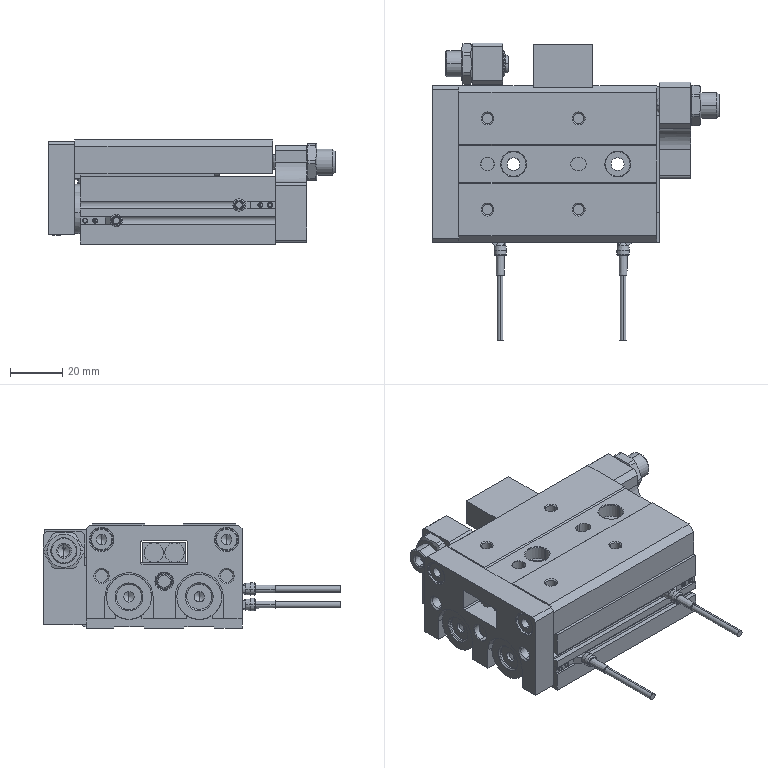Part | SolidWorks | features BaseBody 4, MoveFace 1 | 4 solids | 733 faces | box 110 x 114.42 x 40 mm | volume 193406 mm3 | plane 285 | cylinder 262 | cone 146 | spline 36 | torus 4 | commonest cylinder face diameters 4.134 x28 7.5 x20 16 x17 9 x16 4 x12 8.5 x12